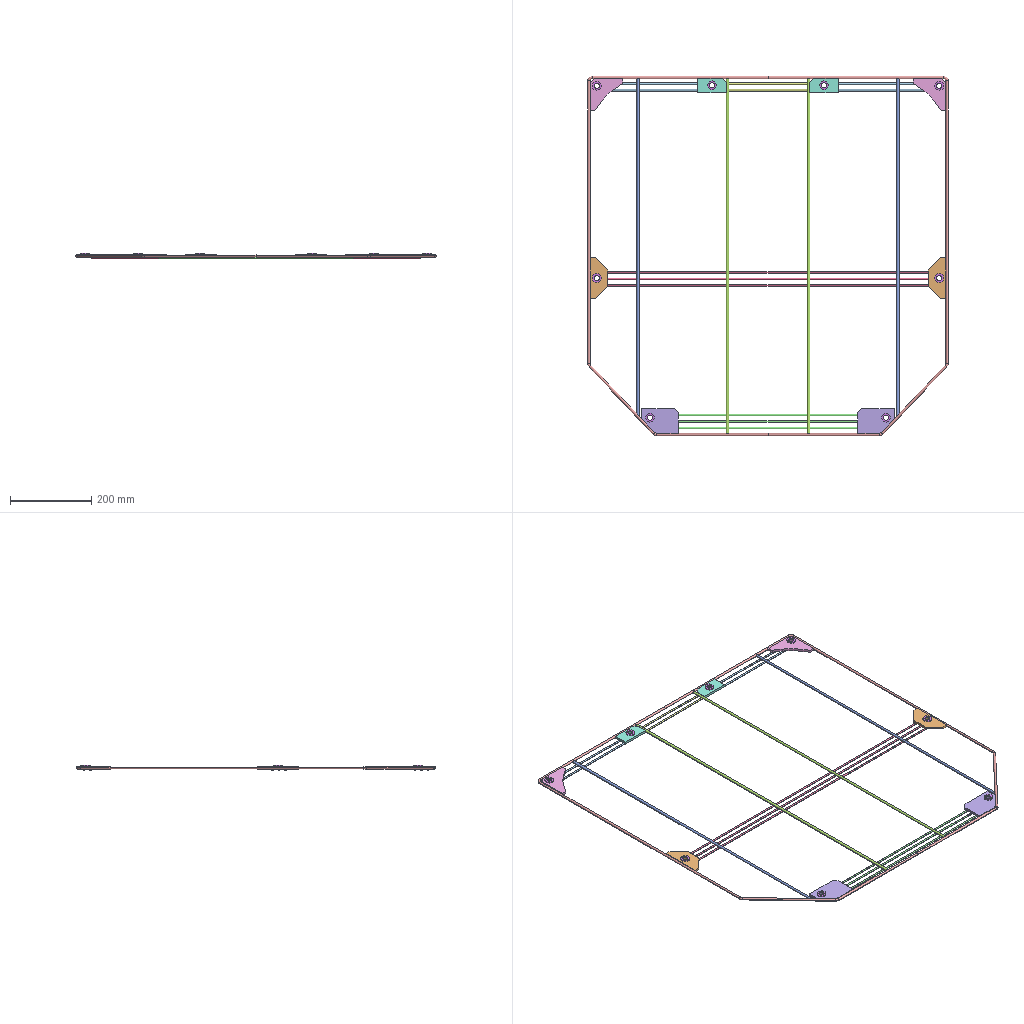Assembly | SolidWorks | 12 different items | 34 placed | box 889 x 887 x 13 mm
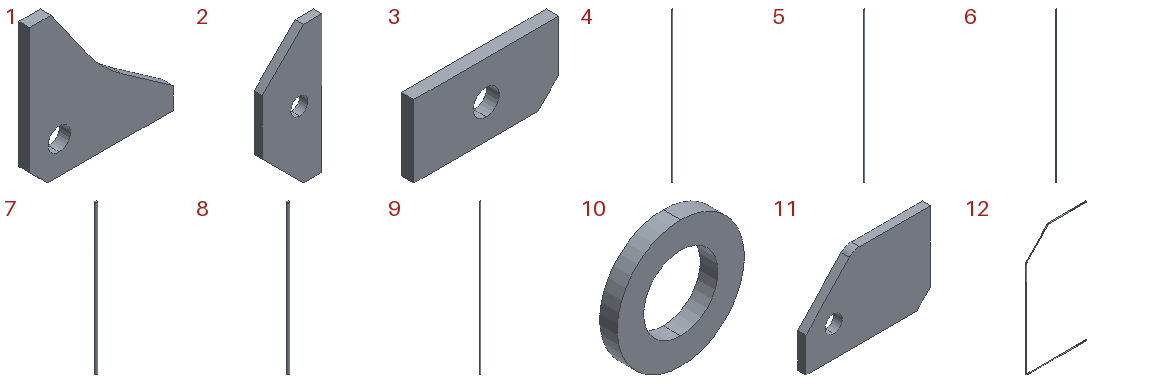Parts list (item | quantity | size | volume | features):
1 | x2 | 80 x 6 x 80 mm | 21113 mm3 | features FlatPattern 1, SMBaseFlange 1, SheetMetal 1
2 | x2 | 43.5 x 6 x 100 mm | 19964 mm3 | features FlatPattern 1, SMBaseFlange 1, SheetMetal 1
3 | x2 | 70 x 6 x 35 mm | 13664 mm3 | features FlatPattern 1, SMBaseFlange 1, SheetMetal 1
4 | x2 | 6 x 6 x 832.8 mm | 23463 mm3 | features Extrusion 1, ICE 1
5 | x3 | 4 x 4 x 479.4 mm | 6024 mm3 | features Extrusion 1
6 | x3 | 4 x 4 x 810 mm | 10179 mm3 | features Extrusion 1
7 | x4 | 4 x 4 x 242.5 mm | 3047 mm3 | features Extrusion 1
8 | x2 | 4 x 4 x 236 mm | 2966 mm3 | features Extrusion 1
9 | x2 | 6 x 6 x 875 mm | 24740 mm3 | features Extrusion 1
10 | x8 | 21.7 x 3 x 21.7 mm | 729.478 mm3 | features FlatPattern 1, SMBaseFlange 1, SheetMetal 1
11 | x2 | 90 x 6 x 61.1 mm | 28229 mm3 | features FlatPattern 1, SMBaseFlange 1, SheetMetal 1
12 | x2 | 444.5 x 6 x 887 mm | 46970 mm3 | features Sweep 1
Mates (type | each side: item.copy, entity, surface, feature):
Coincident | 12.1 edge | 12.2 edge | 2 times
Tangent | 12.1 face cylinder Sweep1 | 4.1 face plane Boss-Extrude1
DistanceDim | 12.1 face cylinder Sweep1 | 4.1 face cylinder Boss-Extrude1
Parallel | 12.1 face cylinder Sweep1 | 4.1 face cylinder Boss-Extrude1
Parallel | 12.1 plane | 4.1 plane
Coincident | 12.1 plane | 4.1 plane
Coincident | 12.1 plane | 9.1 plane
Tangent | 12.1 face cylinder Sweep1 | 9.1 face plane Boss-Extrude1
DistanceDim | 9.1 plane | 4.1 plane
DistanceDim | 12.1 plane | 1.1 face plane Base-Flange1
Tangent | 12.1 face cylinder Sweep1 | 1.1 face plane Base-Flange1 | 2 times
Coincident | 1.1 face plane Base-Flange1 | 3.1 face plane Base-Flange1
Tangent | 12.1 face cylinder Sweep1 | 3.1 face plane Base-Flange1
Tangent | 9.1 face cylinder Boss-Extrude1 | 3.1 face plane Base-Flange1
Coincident | 1.1 face plane Base-Flange1 | 2.1 face plane Base-Flange1
Tangent | 12.1 face cylinder Sweep1 | 2.1 face plane Base-Flange1
DistanceDim | 1.1 face cylinder Base-Flange1 | 2.1 face cylinder Base-Flange1
Coincident | 2.1 face plane Base-Flange1 | 11.1 face plane Base-Flange1
Tangent | 12.1 face cylinder Sweep1 | 11.1 face plane Base-Flange1
DistanceDim | 2.1 face plane Base-Flange1 | 11.1 face plane Base-Flange1
Coincident | 12.1 plane | 4.2 plane
DistanceDim | 4.2 plane | 12.1 plane
Tangent | 12.2 face cylinder Sweep1 | 4.2 face plane Boss-Extrude1
DistanceDim | 5.1 plane | 11.2 face plane Base-Flange1
DistanceDim | 5.1 face plane Boss-Extrude1 | 12.1 face cylinder Sweep1
DistanceDim | 5.1 face cylinder Boss-Extrude1 | 12.2 face cylinder Sweep1
DistanceDim | 6.1 plane | 2.1 face plane Base-Flange1
DistanceDim | 6.1 face plane Boss-Extrude1 | 12.1 face cylinder Sweep1
DistanceDim | 6.1 plane | 5.1 plane
DistanceDim | 7.1 plane | 3.2 face plane Base-Flange1
DistanceDim | 3.2 face plane Base-Flange1 | 7.1 face plane Boss-Extrude1
DistanceDim | 7.1 plane | 12.1 plane
Concentric | 7.1 face cylinder Boss-Extrude1 | 8.1 face cylinder Boss-Extrude1
DistanceDim | 3.1 face plane Base-Flange1 | 8.1 face plane Boss-Extrude1
Parallel | 3.1 face plane Base-Flange1 | 8.1 plane
Coincident | 1.1 face plane Base-Flange1 | 10.1 face plane Base-Flange1
Concentric | 1.1 face cylinder Base-Flange1 | 10.1 face cylinder Base-Flange1
Parallel | 1.1 face plane Base-Flange1 | 10.1 plane
Coincident | 3.1 face plane Base-Flange1 | 10.2 face plane Base-Flange1
Concentric | 3.1 face cylinder Base-Flange1 | 10.2 face cylinder Base-Flange1
Coincident | 2.1 face plane Base-Flange1 | 10.3 face plane Base-Flange1
Concentric | 2.1 face cylinder Base-Flange1 | 10.3 face cylinder Base-Flange1
Concentric | 11.1 face cylinder Base-Flange1 | 10.4 face cylinder Base-Flange1
Coincident | 11.1 face plane Base-Flange1 | 10.4 face plane Base-Flange1